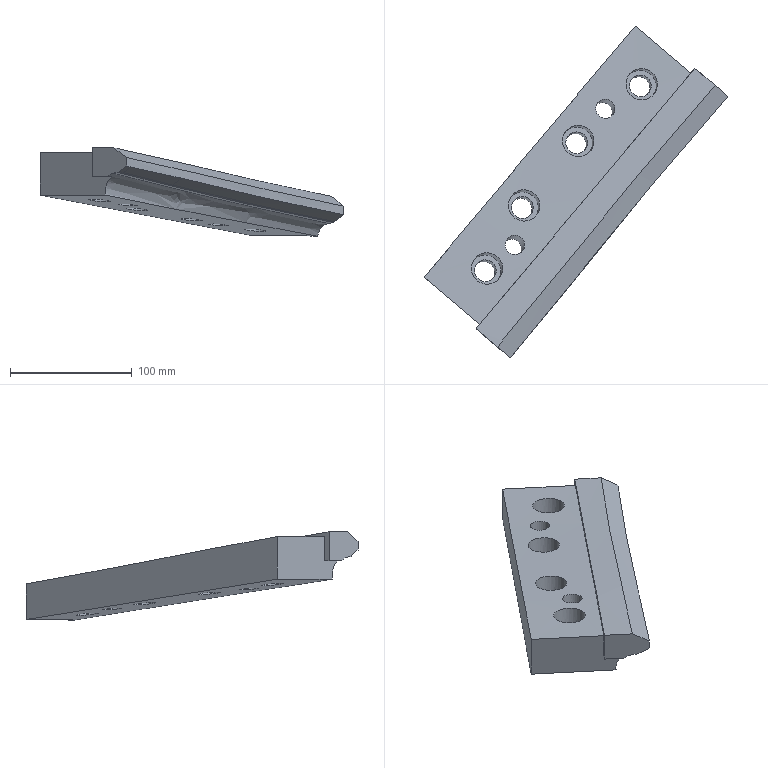Part | NX | features solid 2 | 1 solid | 34 faces | box 249.975 x 273.072 x 72.736 mm | volume 684487 mm3 | plane 12 | spline 12 | cylinder 10 | commonest cylinder face diameters 18 x4 26 x4 16 x2